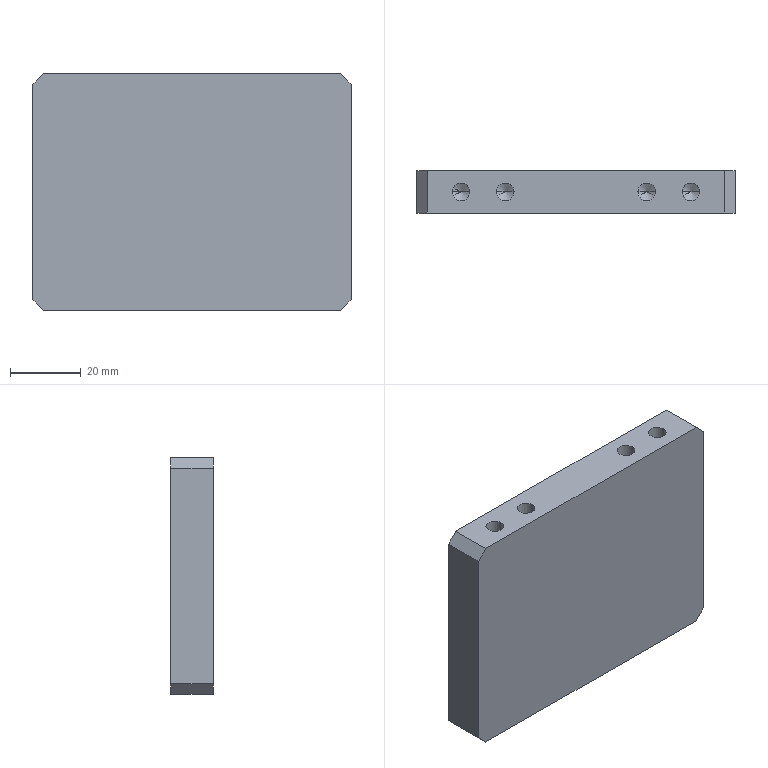Part | STEP file | PN_0065 | 1 solid | 42 faces | box 90 x 12 x 67 mm | volume 69945 mm3 | cylinder 16 | cone 16 | plane 10 | commonest cylinder face diameters 5 x16